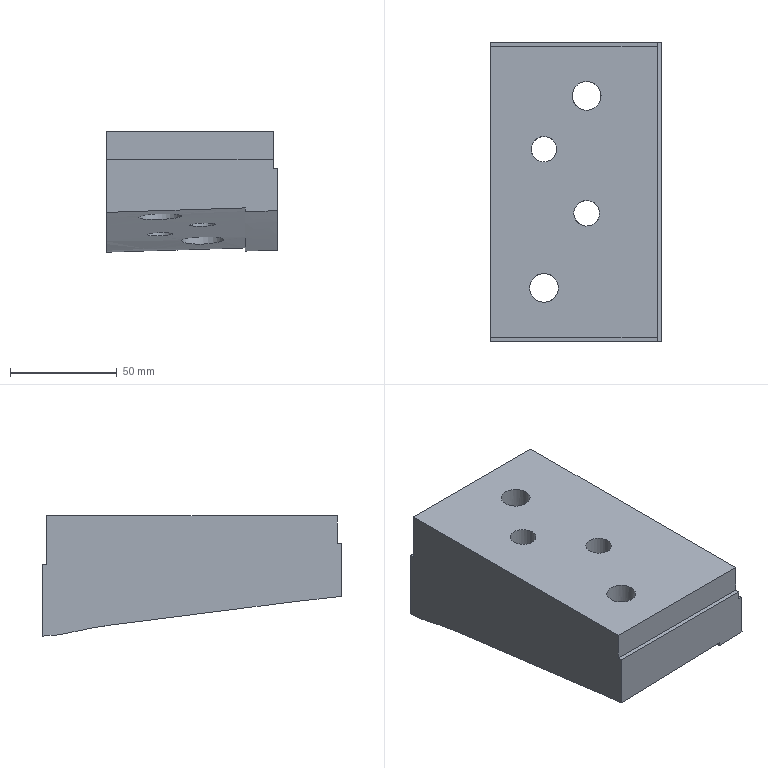Part | NX | features solid 2 | 1 solid | 22 faces | box 80 x 140 x 56.387 mm | volume 462512 mm3 | plane 9 | spline 7 | cylinder 6 | commonest cylinder face diameters 12 x2 13.5 x2 20 x2
STEP:
#1=CARTESIAN_POINT('',(-340.604,272.143,-48.935));
#2=VERTEX_POINT('',#1);
#3=CARTESIAN_POINT('',(-337.704,276.084,-49.337));
#4=CARTESIAN_POINT('',(-341.213,272.366,-48.983));
#5=CARTESIAN_POINT('',(-341.071,267.308,-48.342));
#6=CARTESIAN_POINT('',(-337.412,263.802,-47.781));
#7=CARTESIAN_POINT('',(-332.295,263.917,-47.63));
#8=CARTESIAN_POINT('',(-328.79,267.632,-47.987));
#9=CARTESIAN_POINT('',(-328.926,272.684,-48.627));
#10=CARTESIAN_POINT('',(-332.584,276.197,-49.186));
#11=CARTESIAN_POINT('',(-337.704,276.084,-49.337));
#12=CARTESIAN_POINT('',(-341.213,272.366,-48.983));
#13=CARTESIAN_POINT('',(-341.071,267.308,-48.342));
#14=B_SPLINE_CURVE_WITH_KNOTS('',3,(#3,#4,#5,#6,#7,#8,#9,#10,#11,#12,#13),.UNSPECIFIED.,.T.,.F.,(1,1,1,1,1,1,1,1,1,1,1,1,1,1,1),(-0.01413,-0.009417,-0.004708,0.,0.004708,0.009417,0.01413,0.01883,0.02354,0.02825,0.03296,0.03767,0.04238,0.04708,0.05179),.UNSPECIFIED.);
#15=EDGE_CURVE('',#2,#2,#14,.T.);
#16=ORIENTED_EDGE('',*,*,#15,.T.);
#17=EDGE_LOOP('',(#16));
#18=FACE_BOUND('',#17,.T.);
#19=CARTESIAN_POINT('',(-364.93,233.823,-44.972));
#20=VERTEX_POINT('',#19);
#21=CARTESIAN_POINT('',(-361.894,226.328,-43.775));
#22=CARTESIAN_POINT('',(-365.992,233.692,-45.025));
#23=CARTESIAN_POINT('',(-363.722,241.842,-45.959));
#24=CARTESIAN_POINT('',(-356.292,246.019,-46.2));
#25=CARTESIAN_POINT('',(-348.103,243.675,-45.634));
#26=CARTESIAN_POINT('',(-344.008,236.287,-44.614));
#27=CARTESIAN_POINT('',(-346.274,228.169,-43.516));
#28=CARTESIAN_POINT('',(-353.707,223.978,-43.211));
#29=CARTESIAN_POINT('',(-361.894,226.328,-43.775));
#30=CARTESIAN_POINT('',(-365.992,233.692,-45.025));
#31=CARTESIAN_POINT('',(-363.722,241.842,-45.959));
#32=B_SPLINE_CURVE_WITH_KNOTS('',3,(#21,#22,#23,#24,#25,#26,#27,#28,#29,#30,#31),.UNSPECIFIED.,.T.,.F.,(1,1,1,1,1,1,1,1,1,1,1,1,1,1,1),(-0.02356,-0.0157,-0.007852,0.,0.007852,0.0157,0.02356,0.03141,0.03926,0.04711,0.05496,0.06281,0.07067,0.07852,0.08637),.UNSPECIFIED.);
#33=EDGE_CURVE('',#20,#20,#32,.T.);
#34=ORIENTED_EDGE('',*,*,#33,.F.);
#35=EDGE_LOOP('',(#34));
#36=FACE_BOUND('',#35,.T.);
#37=CARTESIAN_POINT('',(-314.991,210.,-40.636));
#38=VERTEX_POINT('',#37);
#39=CARTESIAN_POINT('',(-380.,210.,-42.734));
#40=VERTEX_POINT('',#39);
#41=CARTESIAN_POINT('',(-314.991,210.,-40.636));
#42=CARTESIAN_POINT('',(-336.664,210.,-41.245));
#43=CARTESIAN_POINT('',(-358.334,210.,-41.928));
#44=CARTESIAN_POINT('',(-380.,210.,-42.734));
#45=B_SPLINE_CURVE_WITH_KNOTS('',3,(#41,#42,#43,#44),.UNSPECIFIED.,.F.,.F.,(4,4),(0.01025,0.07529),.UNSPECIFIED.);
#46=EDGE_CURVE('',#38,#40,#45,.T.);
#47=ORIENTED_EDGE('',*,*,#46,.T.);
#48=CARTESIAN_POINT('',(-380.,350.,-61.387));
#49=VERTEX_POINT('',#48);
#50=CARTESIAN_POINT('',(-380.,210.,-42.734));
#51=CARTESIAN_POINT('',(-380.,212.923,-43.037));
#52=CARTESIAN_POINT('',(-380.,218.777,-43.562));
#53=CARTESIAN_POINT('',(-380.,227.539,-44.553));
#54=CARTESIAN_POINT('',(-380.,236.272,-45.886));
#55=CARTESIAN_POINT('',(-380.,245.041,-46.917));
#56=CARTESIAN_POINT('',(-380.,253.807,-47.989));
#57=CARTESIAN_POINT('',(-380.,265.486,-49.471));
#58=CARTESIAN_POINT('',(-380.,280.086,-51.318));
#59=CARTESIAN_POINT('',(-380.,294.685,-53.165));
#60=CARTESIAN_POINT('',(-380.,306.364,-54.652));
#61=CARTESIAN_POINT('',(-380.,315.123,-55.762));
#62=CARTESIAN_POINT('',(-380.,323.875,-56.931));
#63=CARTESIAN_POINT('',(-380.,332.562,-58.574));
#64=CARTESIAN_POINT('',(-380.,341.152,-60.922));
#65=CARTESIAN_POINT('',(-380.,347.062,-61.148));
#66=CARTESIAN_POINT('',(-380.,350.,-61.387));
#67=B_SPLINE_CURVE_WITH_KNOTS('',3,(#50,#51,#52,#53,#54,#55,#56,#57,#58,#59,#60,#61,#62,#63,#64,#65,#66),.UNSPECIFIED.,.F.,.F.,(4,1,1,1,1,1,1,1,1,1,1,1,1,1,4),(0.1253,0.1342,0.143,0.1518,0.1606,0.1694,0.1782,0.1959,0.2135,0.2223,0.2311,0.2399,0.2488,0.2576,0.2664),.UNSPECIFIED.);
#68=EDGE_CURVE('',#40,#49,#67,.T.);
#69=ORIENTED_EDGE('',*,*,#68,.T.);
#70=CARTESIAN_POINT('',(-314.998,350.,-59.39));
#71=VERTEX_POINT('',#70);
#72=CARTESIAN_POINT('',(-314.998,350.,-59.39));
#73=CARTESIAN_POINT('',(-336.667,350.,-59.991));
#74=CARTESIAN_POINT('',(-358.334,350.,-60.686));
#75=CARTESIAN_POINT('',(-380.,350.,-61.387));
#76=B_SPLINE_CURVE_WITH_KNOTS('',3,(#72,#73,#74,#75),.UNSPECIFIED.,.F.,.F.,(4,4),(-0.01501,0.05002),.UNSPECIFIED.);
#77=EDGE_CURVE('',#71,#49,#76,.T.);
#78=ORIENTED_EDGE('',*,*,#77,.F.);
#79=CARTESIAN_POINT('',(-314.998,350.,-59.39));
#80=CARTESIAN_POINT('',(-314.996,347.092,-58.943));
#81=CARTESIAN_POINT('',(-314.993,341.269,-58.09));
#82=CARTESIAN_POINT('',(-314.99,332.599,-56.409));
#83=CARTESIAN_POINT('',(-314.988,323.924,-54.761));
#84=CARTESIAN_POINT('',(-314.986,315.176,-53.571));
#85=CARTESIAN_POINT('',(-314.985,306.414,-52.466));
#86=CARTESIAN_POINT('',(-314.983,294.733,-50.983));
#87=CARTESIAN_POINT('',(-314.983,280.132,-49.135));
#88=CARTESIAN_POINT('',(-314.984,262.608,-46.929));
#89=CARTESIAN_POINT('',(-314.985,248.007,-45.079));
#90=CARTESIAN_POINT('',(-314.987,236.316,-43.671));
#91=CARTESIAN_POINT('',(-314.988,227.574,-42.418));
#92=CARTESIAN_POINT('',(-314.99,218.799,-41.409));
#93=CARTESIAN_POINT('',(-314.991,212.932,-40.901));
#94=CARTESIAN_POINT('',(-314.991,210.,-40.636));
#95=B_SPLINE_CURVE_WITH_KNOTS('',3,(#79,#80,#81,#82,#83,#84,#85,#86,#87,#88,#89,#90,#91,#92,#93,#94),.UNSPECIFIED.,.F.,.F.,(4,1,1,1,1,1,1,1,1,1,1,1,1,4),(0.,0.008827,0.01765,0.02648,0.03531,0.04413,0.05296,0.07061,0.08827,0.1059,0.1147,0.1236,0.1324,0.1412),.UNSPECIFIED.);
#96=EDGE_CURVE('',#71,#38,#95,.T.);
#97=ORIENTED_EDGE('',*,*,#96,.T.);
#98=EDGE_LOOP('',(#47,#69,#78,#97));
#99=FACE_BOUND('',#98,.T.);
#100=CARTESIAN_POINT('',(-360.605,302.142,-53.408));
#101=VERTEX_POINT('',#100);
#102=CARTESIAN_POINT('',(-357.705,306.084,-53.808));
#103=CARTESIAN_POINT('',(-361.213,302.365,-53.457));
#104=CARTESIAN_POINT('',(-361.07,297.307,-52.812));
#105=CARTESIAN_POINT('',(-357.411,293.802,-52.241));
#106=CARTESIAN_POINT('',(-352.295,293.917,-52.079));
#107=CARTESIAN_POINT('',(-348.789,297.634,-52.43));
#108=CARTESIAN_POINT('',(-348.927,302.686,-53.074));
#109=CARTESIAN_POINT('',(-352.585,306.197,-53.646));
#110=CARTESIAN_POINT('',(-357.705,306.084,-53.808));
#111=CARTESIAN_POINT('',(-361.213,302.365,-53.457));
#112=CARTESIAN_POINT('',(-361.07,297.307,-52.812));
#113=B_SPLINE_CURVE_WITH_KNOTS('',3,(#102,#103,#104,#105,#106,#107,#108,#109,#110,#111,#112),.UNSPECIFIED.,.T.,.F.,(1,1,1,1,1,1,1,1,1,1,1,1,1,1,1),(-0.01413,-0.009418,-0.004709,0.,0.004709,0.009418,0.01413,0.01884,0.02354,0.02825,0.03296,0.03767,0.04238,0.04709,0.0518),.UNSPECIFIED.);
#114=EDGE_CURVE('',#101,#101,#113,.T.);
#115=ORIENTED_EDGE('',*,*,#114,.T.);
#116=EDGE_LOOP('',(#115));
#117=FACE_BOUND('',#116,.T.);
#118=CARTESIAN_POINT('',(-325.086,326.305,-55.559));
#119=VERTEX_POINT('',#118);
#120=CARTESIAN_POINT('',(-328.189,333.733,-57.085));
#121=CARTESIAN_POINT('',(-324.036,326.454,-55.489));
#122=CARTESIAN_POINT('',(-326.178,318.281,-54.313));
#123=CARTESIAN_POINT('',(-333.578,313.989,-54.013));
#124=CARTESIAN_POINT('',(-341.824,316.259,-54.566));
#125=CARTESIAN_POINT('',(-345.974,323.624,-55.697));
#126=CARTESIAN_POINT('',(-343.806,331.716,-57.207));
#127=CARTESIAN_POINT('',(-336.422,336.014,-57.861));
#128=CARTESIAN_POINT('',(-328.189,333.733,-57.085));
#129=CARTESIAN_POINT('',(-324.036,326.454,-55.489));
#130=CARTESIAN_POINT('',(-326.178,318.281,-54.313));
#131=B_SPLINE_CURVE_WITH_KNOTS('',3,(#120,#121,#122,#123,#124,#125,#126,#127,#128,#129,#130),.UNSPECIFIED.,.T.,.F.,(1,1,1,1,1,1,1,1,1,1,1,1,1,1,1),(-0.02362,-0.01575,-0.007874,0.,0.007874,0.01575,0.02362,0.0315,0.03937,0.04725,0.05512,0.063,0.07087,0.07874,0.08662),.UNSPECIFIED.);
#132=EDGE_CURVE('',#119,#119,#131,.T.);
#133=ORIENTED_EDGE('',*,*,#132,.F.);
#134=EDGE_LOOP('',(#133));
#135=FACE_BOUND('',#134,.T.);
#136=CARTESIAN_POINT('',(-300.962,350.,-59.01));
#137=CARTESIAN_POINT('',(-301.431,346.762,-58.489));
#138=CARTESIAN_POINT('',(-302.299,340.897,-57.565));
#139=CARTESIAN_POINT('',(-303.25,332.345,-55.971));
#140=CARTESIAN_POINT('',(-304.418,323.079,-54.303));
#141=CARTESIAN_POINT('',(-305.393,313.774,-53.112));
#142=CARTESIAN_POINT('',(-306.505,303.143,-51.799));
#143=CARTESIAN_POINT('',(-307.441,293.837,-50.646));
#144=CARTESIAN_POINT('',(-308.479,283.202,-49.331));
#145=CARTESIAN_POINT('',(-309.382,273.894,-48.18));
#146=CARTESIAN_POINT('',(-310.372,263.256,-46.87));
#147=CARTESIAN_POINT('',(-311.258,253.944,-45.722));
#148=CARTESIAN_POINT('',(-312.072,243.308,-44.419));
#149=CARTESIAN_POINT('',(-312.85,233.989,-43.303));
#150=CARTESIAN_POINT('',(-313.651,223.335,-41.796));
#151=CARTESIAN_POINT('',(-314.257,215.772,-41.146));
#152=CARTESIAN_POINT('',(-314.465,210.889,-40.701));
#153=CARTESIAN_POINT('',(-314.5,210.,-40.622));
#154=CARTESIAN_POINT('',(-314.02,350.,-59.356));
#155=CARTESIAN_POINT('',(-314.503,346.762,-58.865));
#156=CARTESIAN_POINT('',(-315.396,340.897,-58.023));
#157=CARTESIAN_POINT('',(-316.39,332.345,-56.402));
#158=CARTESIAN_POINT('',(-317.606,323.079,-54.671));
#159=CARTESIAN_POINT('',(-318.618,313.774,-53.501));
#160=CARTESIAN_POINT('',(-319.775,303.143,-52.185));
#161=CARTESIAN_POINT('',(-320.748,293.837,-51.037));
#162=CARTESIAN_POINT('',(-321.828,283.202,-49.725));
#163=CARTESIAN_POINT('',(-322.766,273.894,-48.577));
#164=CARTESIAN_POINT('',(-323.796,263.256,-47.271));
#165=CARTESIAN_POINT('',(-324.709,253.944,-46.126));
#166=CARTESIAN_POINT('',(-325.587,243.308,-44.837));
#167=CARTESIAN_POINT('',(-326.387,233.989,-43.734));
#168=CARTESIAN_POINT('',(-327.225,223.335,-42.178));
#169=CARTESIAN_POINT('',(-327.854,215.772,-41.548));
#170=CARTESIAN_POINT('',(-328.077,210.889,-41.086));
#171=CARTESIAN_POINT('',(-328.115,210.,-41.004));
#172=CARTESIAN_POINT('',(-340.52,350.,-60.099));
#173=CARTESIAN_POINT('',(-341.03,346.762,-59.688));
#174=CARTESIAN_POINT('',(-341.969,340.897,-59.065));
#175=CARTESIAN_POINT('',(-343.058,332.345,-57.312));
#176=CARTESIAN_POINT('',(-344.37,323.079,-55.476));
#177=CARTESIAN_POINT('',(-345.46,313.774,-54.346));
#178=CARTESIAN_POINT('',(-346.706,303.143,-53.023));
#179=CARTESIAN_POINT('',(-347.754,293.837,-51.885));
#180=CARTESIAN_POINT('',(-348.919,283.202,-50.579));
#181=CARTESIAN_POINT('',(-349.928,273.894,-49.435));
#182=CARTESIAN_POINT('',(-351.041,263.256,-48.137));
#183=CARTESIAN_POINT('',(-352.009,253.944,-46.994));
#184=CARTESIAN_POINT('',(-353.015,243.308,-45.734));
#185=CARTESIAN_POINT('',(-353.86,233.989,-44.657));
#186=CARTESIAN_POINT('',(-354.774,223.335,-43.011));
#187=CARTESIAN_POINT('',(-355.446,215.772,-42.425));
#188=CARTESIAN_POINT('',(-355.703,210.889,-41.926));
#189=CARTESIAN_POINT('',(-355.748,210.,-41.838));
#190=CARTESIAN_POINT('',(-367.021,350.,-60.967));
#191=CARTESIAN_POINT('',(-367.548,346.762,-60.703));
#192=CARTESIAN_POINT('',(-368.502,340.897,-60.466));
#193=CARTESIAN_POINT('',(-369.739,332.345,-58.166));
#194=CARTESIAN_POINT('',(-371.126,323.079,-56.442));
#195=CARTESIAN_POINT('',(-372.298,313.774,-55.304));
#196=CARTESIAN_POINT('',(-373.633,303.143,-53.988));
#197=CARTESIAN_POINT('',(-374.757,293.837,-52.856));
#198=CARTESIAN_POINT('',(-376.006,283.202,-51.554));
#199=CARTESIAN_POINT('',(-377.086,273.894,-50.413));
#200=CARTESIAN_POINT('',(-378.28,263.256,-49.117));
#201=CARTESIAN_POINT('',(-379.311,253.944,-47.967));
#202=CARTESIAN_POINT('',(-380.416,243.308,-46.721));
#203=CARTESIAN_POINT('',(-381.319,233.989,-45.631));
#204=CARTESIAN_POINT('',(-382.302,223.335,-44.011));
#205=CARTESIAN_POINT('',(-383.015,215.772,-43.446));
#206=CARTESIAN_POINT('',(-383.311,210.889,-42.932));
#207=CARTESIAN_POINT('',(-383.363,210.,-42.841));
#208=CARTESIAN_POINT('',(-380.472,350.,-61.402));
#209=CARTESIAN_POINT('',(-381.011,346.762,-61.156));
#210=CARTESIAN_POINT('',(-381.985,340.897,-60.965));
#211=CARTESIAN_POINT('',(-383.269,332.345,-58.644));
#212=CARTESIAN_POINT('',(-384.699,323.079,-56.959));
#213=CARTESIAN_POINT('',(-385.911,313.774,-55.824));
#214=CARTESIAN_POINT('',(-387.291,303.143,-54.514));
#215=CARTESIAN_POINT('',(-388.453,293.837,-53.383));
#216=CARTESIAN_POINT('',(-389.745,283.202,-52.084));
#217=CARTESIAN_POINT('',(-390.861,273.894,-50.942));
#218=CARTESIAN_POINT('',(-392.096,263.256,-49.645));
#219=CARTESIAN_POINT('',(-393.163,253.944,-48.489));
#220=CARTESIAN_POINT('',(-394.303,243.308,-47.245));
#221=CARTESIAN_POINT('',(-395.243,233.989,-46.127));
#222=CARTESIAN_POINT('',(-396.256,223.335,-44.574));
#223=CARTESIAN_POINT('',(-396.988,215.772,-44.006));
#224=CARTESIAN_POINT('',(-397.308,210.889,-43.498));
#225=CARTESIAN_POINT('',(-397.364,210.,-43.407));
#226=B_SPLINE_SURFACE_WITH_KNOTS('',3,3,((#136,#137,#138,#139,#140,#141,#142,#143,#144,#145,#146,#147,#148,#149,#150,#151,#152,#153),(#154,#155,#156,#157,#158,#159,#160,#161,#162,#163,#164,#165,#166,#167,#168,#169,#170,#171),(#172,#173,#174,#175,#176,#177,#178,#179,#180,#181,#182,#183,#184,#185,#186,#187,#188,#189),(#190,#191,#192,#193,#194,#195,#196,#197,#198,#199,#200,#201,#202,#203,#204,#205,#206,#207),(#208,#209,#210,#211,#212,#213,#214,#215,#216,#217,#218,#219,#220,#221,#222,#223,#224,#225)),.UNSPECIFIED.,.F.,.F.,.F.,(4,1,4),(4,1,1,1,1,1,1,1,1,1,1,1,1,1,1,4),(0.7767,0.8125,0.8494),(0.2465,0.2656,0.2812,0.2969,0.3203,0.3359,0.3594,0.375,0.3984,0.4141,0.4375,0.4531,0.4766,0.4922,0.5156,0.5208),.UNSPECIFIED.);
#227=ADVANCED_FACE('',(#18,#36,#99,#117,#135),#226,.F.);
#228=CARTESIAN_POINT('',(-302.,348.,-28.));
#229=VERTEX_POINT('',#228);
#230=CARTESIAN_POINT('',(-380.,348.,-28.));
#231=VERTEX_POINT('',#230);
#232=CARTESIAN_POINT('',(-302.,348.,-28.));
#233=DIRECTION('',(1.,0.,0.));
#234=VECTOR('',#233,1000.);
#235=LINE('',#232,#234);
#236=EDGE_CURVE('',#229,#231,#235,.F.);
#237=ORIENTED_EDGE('',*,*,#236,.F.);
#238=CARTESIAN_POINT('',(-302.,350.,-28.));
#239=VERTEX_POINT('',#238);
#240=CARTESIAN_POINT('',(-302.,350.,-28.));
#241=DIRECTION('',(0.,1.,0.));
#242=VECTOR('',#241,1000.);
#243=LINE('',#240,#242);
#244=EDGE_CURVE('',#239,#229,#243,.F.);
#245=ORIENTED_EDGE('',*,*,#244,.F.);
#246=CARTESIAN_POINT('',(-380.,350.,-28.));
#247=VERTEX_POINT('',#246);
#248=CARTESIAN_POINT('',(-302.,350.,-28.));
#249=DIRECTION('',(1.,0.,0.));
#250=VECTOR('',#249,1000.);
#251=LINE('',#248,#250);
#252=EDGE_CURVE('',#239,#247,#251,.F.);
#253=ORIENTED_EDGE('',*,*,#252,.T.);
#254=CARTESIAN_POINT('',(-380.,350.,-28.));
#255=DIRECTION('',(0.,1.,0.));
#256=VECTOR('',#255,1000.);
#257=LINE('',#254,#256);
#258=EDGE_CURVE('',#247,#231,#257,.F.);
#259=ORIENTED_EDGE('',*,*,#258,.T.);
#260=EDGE_LOOP('',(#237,#245,#253,#259));
#261=FACE_BOUND('',#260,.T.);
#262=CARTESIAN_POINT('',(-302.,350.,-28.));
#263=DIRECTION('',(0.,0.,1.));
#264=DIRECTION('',(1.,0.,0.));
#265=AXIS2_PLACEMENT_3D('',#262,#263,#264);
#266=PLANE('',#265);
#267=ADVANCED_FACE('',(#261),#266,.T.);
#268=CARTESIAN_POINT('',(-380.,350.,-61.387));
#269=CARTESIAN_POINT('',(-380.,350.,-50.258));
#270=CARTESIAN_POINT('',(-380.,350.,-39.129));
#271=CARTESIAN_POINT('',(-380.,350.,-28.));
#272=B_SPLINE_CURVE_WITH_KNOTS('',3,(#268,#269,#270,#271),.UNSPECIFIED.,.F.,.F.,(4,4),(0.,0.03339),.UNSPECIFIED.);
#273=EDGE_CURVE('',#49,#247,#272,.T.);
#274=ORIENTED_EDGE('',*,*,#273,.T.);
#275=ORIENTED_EDGE('',*,*,#252,.F.);
#276=CARTESIAN_POINT('',(-302.,350.,-40.416));
#277=VERTEX_POINT('',#276);
#278=CARTESIAN_POINT('',(-302.,350.,-40.416));
#279=DIRECTION('',(0.,0.,1.));
#280=VECTOR('',#279,1000.);
#281=LINE('',#278,#280);
#282=EDGE_CURVE('',#277,#239,#281,.T.);
#283=ORIENTED_EDGE('',*,*,#282,.F.);
#284=CARTESIAN_POINT('',(-300.,350.,-40.416));
#285=VERTEX_POINT('',#284);
#286=CARTESIAN_POINT('',(-302.,350.,-40.416));
#287=CARTESIAN_POINT('',(-301.333,350.,-40.416));
#288=CARTESIAN_POINT('',(-300.667,350.,-40.416));
#289=CARTESIAN_POINT('',(-300.,350.,-40.416));
#290=B_SPLINE_CURVE_WITH_KNOTS('',3,(#286,#287,#288,#289),.UNSPECIFIED.,.F.,.F.,(4,4),(0.,1.),.UNSPECIFIED.);
#291=EDGE_CURVE('',#285,#277,#290,.F.);
#292=ORIENTED_EDGE('',*,*,#291,.F.);
#293=CARTESIAN_POINT('',(-300.,350.,-60.416));
#294=VERTEX_POINT('',#293);
#295=CARTESIAN_POINT('',(-300.,350.,-38.122));
#296=DIRECTION('',(0.,0.,1.));
#297=VECTOR('',#296,1000.);
#298=LINE('',#295,#297);
#299=EDGE_CURVE('',#294,#285,#298,.T.);
#300=ORIENTED_EDGE('',*,*,#299,.F.);
#301=CARTESIAN_POINT('',(-314.998,350.,-60.862));
#302=VERTEX_POINT('',#301);
#303=CARTESIAN_POINT('',(-314.998,350.,-60.862));
#304=CARTESIAN_POINT('',(-309.999,350.,-60.709));
#305=CARTESIAN_POINT('',(-304.999,350.,-60.561));
#306=CARTESIAN_POINT('',(-300.,350.,-60.416));
#307=B_SPLINE_CURVE_WITH_KNOTS('',3,(#303,#304,#305,#306),.UNSPECIFIED.,.F.,.F.,(4,4),(0.02527,0.04027),.UNSPECIFIED.);
#308=EDGE_CURVE('',#302,#294,#307,.T.);
#309=ORIENTED_EDGE('',*,*,#308,.F.);
#310=CARTESIAN_POINT('',(-314.998,350.,-96.));
#311=DIRECTION('',(0.,0.,1.));
#312=VECTOR('',#311,1000.);
#313=LINE('',#310,#312);
#314=EDGE_CURVE('',#302,#71,#313,.T.);
#315=ORIENTED_EDGE('',*,*,#314,.T.);
#316=ORIENTED_EDGE('',*,*,#77,.T.);
#317=EDGE_LOOP('',(#274,#275,#283,#292,#300,#309,#315,#316));
#318=FACE_BOUND('',#317,.T.);
#319=CARTESIAN_POINT('',(440.921,350.,-40.306));
#320=DIRECTION('',(0.,1.,0.));
#321=DIRECTION('',(0.,0.,1.));
#322=AXIS2_PLACEMENT_3D('',#319,#320,#321);
#323=PLANE('',#322);
#324=ADVANCED_FACE('',(#318),#323,.T.);
#325=CARTESIAN_POINT('',(-302.,348.,-5.));
#326=VERTEX_POINT('',#325);
#327=CARTESIAN_POINT('',(-302.,348.,12.));
#328=DIRECTION('',(0.,0.,1.));
#329=VECTOR('',#328,1000.);
#330=LINE('',#327,#329);
#331=EDGE_CURVE('',#326,#229,#330,.F.);
#332=ORIENTED_EDGE('',*,*,#331,.T.);
#333=ORIENTED_EDGE('',*,*,#236,.T.);
#334=CARTESIAN_POINT('',(-380.,348.,-5.));
#335=VERTEX_POINT('',#334);
#336=CARTESIAN_POINT('',(-380.,348.,12.));
#337=DIRECTION('',(0.,0.,1.));
#338=VECTOR('',#337,1000.);
#339=LINE('',#336,#338);
#340=EDGE_CURVE('',#335,#231,#339,.F.);
#341=ORIENTED_EDGE('',*,*,#340,.F.);
#342=CARTESIAN_POINT('',(-302.,348.,-5.));
#343=DIRECTION('',(-1.,0.,0.));
#344=VECTOR('',#343,1000.);
#345=LINE('',#342,#344);
#346=EDGE_CURVE('',#326,#335,#345,.T.);
#347=ORIENTED_EDGE('',*,*,#346,.F.);
#348=EDGE_LOOP('',(#332,#333,#341,#347));
#349=FACE_BOUND('',#348,.T.);
#350=CARTESIAN_POINT('',(-302.,348.,12.));
#351=DIRECTION('',(0.,1.,0.));
#352=DIRECTION('',(-1.,0.,0.));
#353=AXIS2_PLACEMENT_3D('',#350,#351,#352);
#354=PLANE('',#353);
#355=ADVANCED_FACE('',(#349),#354,.T.);
#356=CARTESIAN_POINT('',(-329.,270.,-5.));
#357=VERTEX_POINT('',#356);
#358=CARTESIAN_POINT('',(-335.,270.,-5.));
#359=DIRECTION('',(0.,0.,1.));
#360=DIRECTION('',(1.,0.,0.));
#361=AXIS2_PLACEMENT_3D('',#358,#359,#360);
#362=CIRCLE('',#361,6.);
#363=EDGE_CURVE('',#357,#357,#362,.F.);
#364=ORIENTED_EDGE('',*,*,#363,.T.);
#365=EDGE_LOOP('',(#364));
#366=FACE_BOUND('',#365,.T.);
#367=CARTESIAN_POINT('',(-341.75,325.,-5.));
#368=VERTEX_POINT('',#367);
#369=CARTESIAN_POINT('',(-335.,325.,-5.));
#370=DIRECTION('',(0.,0.,-1.));
#371=DIRECTION('',(-1.,0.,0.));
#372=AXIS2_PLACEMENT_3D('',#369,#370,#371);
#373=CIRCLE('',#372,6.75);
#374=EDGE_CURVE('',#368,#368,#373,.T.);
#375=ORIENTED_EDGE('',*,*,#374,.T.);
#376=EDGE_LOOP('',(#375));
#377=FACE_BOUND('',#376,.T.);
#378=CARTESIAN_POINT('',(-349.,300.,-5.));
#379=VERTEX_POINT('',#378);
#380=CARTESIAN_POINT('',(-355.,300.,-5.));
#381=DIRECTION('',(0.,0.,1.));
#382=DIRECTION('',(1.,0.,0.));
#383=AXIS2_PLACEMENT_3D('',#380,#381,#382);
#384=CIRCLE('',#383,6.);
#385=EDGE_CURVE('',#379,#379,#384,.F.);
#386=ORIENTED_EDGE('',*,*,#385,.T.);
#387=EDGE_LOOP('',(#386));
#388=FACE_BOUND('',#387,.T.);
#389=CARTESIAN_POINT('',(-361.75,235.,-5.));
#390=VERTEX_POINT('',#389);
#391=CARTESIAN_POINT('',(-355.,235.,-5.));
#392=DIRECTION('',(0.,0.,-1.));
#393=DIRECTION('',(-1.,0.,0.));
#394=AXIS2_PLACEMENT_3D('',#391,#392,#393);
#395=CIRCLE('',#394,6.75);
#396=EDGE_CURVE('',#390,#390,#395,.T.);
#397=ORIENTED_EDGE('',*,*,#396,.T.);
#398=EDGE_LOOP('',(#397));
#399=FACE_BOUND('',#398,.T.);
#400=CARTESIAN_POINT('',(-380.,212.,-5.));
#401=VERTEX_POINT('',#400);
#402=CARTESIAN_POINT('',(-302.,212.,-5.));
#403=VERTEX_POINT('',#402);
#404=CARTESIAN_POINT('',(0.,212.,-5.));
#405=DIRECTION('',(-1.,0.,0.));
#406=VECTOR('',#405,1000.);
#407=LINE('',#404,#406);
#408=EDGE_CURVE('',#401,#403,#407,.F.);
#409=ORIENTED_EDGE('',*,*,#408,.T.);
#410=CARTESIAN_POINT('',(-302.,348.,-5.));
#411=CARTESIAN_POINT('',(-302.,302.667,-5.));
#412=CARTESIAN_POINT('',(-302.,257.333,-5.));
#413=CARTESIAN_POINT('',(-302.,212.,-5.));
#414=B_SPLINE_CURVE_WITH_KNOTS('',3,(#410,#411,#412,#413),.UNSPECIFIED.,.F.,.F.,(4,4),(1.054,1.19),.UNSPECIFIED.);
#415=EDGE_CURVE('',#326,#403,#414,.T.);
#416=ORIENTED_EDGE('',*,*,#415,.F.);
#417=ORIENTED_EDGE('',*,*,#346,.T.);
#418=CARTESIAN_POINT('',(-380.,212.,-5.));
#419=CARTESIAN_POINT('',(-380.,257.333,-5.));
#420=CARTESIAN_POINT('',(-380.,302.667,-5.));
#421=CARTESIAN_POINT('',(-380.,348.,-5.));
#422=B_SPLINE_CURVE_WITH_KNOTS('',3,(#418,#419,#420,#421),.UNSPECIFIED.,.F.,.F.,(4,4),(0.,0.136),.UNSPECIFIED.);
#423=EDGE_CURVE('',#401,#335,#422,.T.);
#424=ORIENTED_EDGE('',*,*,#423,.F.);
#425=EDGE_LOOP('',(#409,#416,#417,#424));
#426=FACE_BOUND('',#425,.T.);
#427=CARTESIAN_POINT('',(0.,0.,-5.));
#428=DIRECTION('',(0.,0.,1.));
#429=DIRECTION('',(-1.,0.,0.));
#430=AXIS2_PLACEMENT_3D('',#427,#428,#429);
#431=PLANE('',#430);
#432=ADVANCED_FACE('',(#366,#377,#388,#399,#426),#431,.T.);
#433=CARTESIAN_POINT('',(-300.,210.,-21.967));
#434=VERTEX_POINT('',#433);
#435=CARTESIAN_POINT('',(-300.,210.,-21.967));
#436=CARTESIAN_POINT('',(-300.,256.574,-26.699));
#437=CARTESIAN_POINT('',(-300.,303.268,-32.848));
#438=CARTESIAN_POINT('',(-300.,350.,-40.416));
#439=B_SPLINE_CURVE_WITH_KNOTS('',3,(#435,#436,#437,#438),.UNSPECIFIED.,.F.,.F.,(4,4),(0.4701,1.),.UNSPECIFIED.);
#440=EDGE_CURVE('',#434,#285,#439,.T.);
#441=ORIENTED_EDGE('',*,*,#440,.T.);
#442=ORIENTED_EDGE('',*,*,#291,.T.);
#443=CARTESIAN_POINT('',(-302.,210.,-21.967));
#444=VERTEX_POINT('',#443);
#445=CARTESIAN_POINT('',(-302.,350.,-40.416));
#446=CARTESIAN_POINT('',(-302.,303.548,-32.894));
#447=CARTESIAN_POINT('',(-302.,256.829,-26.725));
#448=CARTESIAN_POINT('',(-302.,210.,-21.967));
#449=B_SPLINE_CURVE_WITH_KNOTS('',3,(#445,#446,#447,#448),.UNSPECIFIED.,.F.,.F.,(4,4),(0.,0.5298),.UNSPECIFIED.);
#450=EDGE_CURVE('',#444,#277,#449,.F.);
#451=ORIENTED_EDGE('',*,*,#450,.F.);
#452=CARTESIAN_POINT('',(-300.,210.,-21.967));
#453=CARTESIAN_POINT('',(-300.667,210.,-21.967));
#454=CARTESIAN_POINT('',(-301.333,210.,-21.967));
#455=CARTESIAN_POINT('',(-302.,210.,-21.967));
#456=B_SPLINE_CURVE_WITH_KNOTS('',3,(#452,#453,#454,#455),.UNSPECIFIED.,.F.,.F.,(4,4),(0.,0.002),.UNSPECIFIED.);
#457=EDGE_CURVE('',#434,#444,#456,.T.);
#458=ORIENTED_EDGE('',*,*,#457,.F.);
#459=EDGE_LOOP('',(#441,#442,#451,#458));
#460=FACE_BOUND('',#459,.T.);
#461=CARTESIAN_POINT('',(-302.,210.,-21.967));
#462=CARTESIAN_POINT('',(-302.,212.63,-22.234));
#463=CARTESIAN_POINT('',(-302.,215.26,-22.506));
#464=CARTESIAN_POINT('',(-302.,262.074,-27.421));
#465=CARTESIAN_POINT('',(-302.,306.157,-33.316));
#466=CARTESIAN_POINT('',(-302.,350.,-40.416));
#467=CARTESIAN_POINT('',(-300.,210.,-21.967));
#468=CARTESIAN_POINT('',(-300.,212.63,-22.234));
#469=CARTESIAN_POINT('',(-300.,215.26,-22.506));
#470=CARTESIAN_POINT('',(-300.,262.074,-27.421));
#471=CARTESIAN_POINT('',(-300.,306.157,-33.316));
#472=CARTESIAN_POINT('',(-300.,350.,-40.416));
#473=B_SPLINE_SURFACE_WITH_KNOTS('',1,3,((#461,#462,#463,#464,#465,#466),(#467,#468,#469,#470,#471,#472)),.SURF_OF_LINEAR_EXTRUSION.,.F.,.F.,.F.,(2,2),(4,2,4),(0.,1.),(0.4702,0.5,1.),.UNSPECIFIED.);
#474=ADVANCED_FACE('',(#460),#473,.T.);
#475=ORIENTED_EDGE('',*,*,#96,.F.);
#476=ORIENTED_EDGE('',*,*,#314,.F.);
#477=CARTESIAN_POINT('',(-314.991,210.,-42.394));
#478=VERTEX_POINT('',#477);
#479=CARTESIAN_POINT('',(-314.998,350.,-60.862));
#480=CARTESIAN_POINT('',(-314.973,303.523,-53.327));
#481=CARTESIAN_POINT('',(-314.983,256.834,-47.158));
#482=CARTESIAN_POINT('',(-314.991,210.,-42.394));
#483=B_SPLINE_CURVE_WITH_KNOTS('',3,(#479,#480,#481,#482),.UNSPECIFIED.,.F.,.F.,(4,4),(0.,0.1412),.UNSPECIFIED.);
#484=EDGE_CURVE('',#302,#478,#483,.T.);
#485=ORIENTED_EDGE('',*,*,#484,.T.);
#486=CARTESIAN_POINT('',(-314.991,210.,-46.286));
#487=DIRECTION('',(0.,0.,1.));
#488=VECTOR('',#487,1000.);
#489=LINE('',#486,#488);
#490=EDGE_CURVE('',#38,#478,#489,.F.);
#491=ORIENTED_EDGE('',*,*,#490,.F.);
#492=EDGE_LOOP('',(#475,#476,#485,#491));
#493=FACE_BOUND('',#492,.T.);
#494=CARTESIAN_POINT('',(-314.991,210.,-60.983));
#495=CARTESIAN_POINT('',(-314.991,210.,-40.514));
#496=CARTESIAN_POINT('',(-314.991,211.512,-60.983));
#497=CARTESIAN_POINT('',(-314.991,211.512,-40.514));
#498=CARTESIAN_POINT('',(-314.991,213.411,-60.983));
#499=CARTESIAN_POINT('',(-314.991,213.411,-40.514));
#500=CARTESIAN_POINT('',(-314.99,215.673,-60.983));
#501=CARTESIAN_POINT('',(-314.99,215.673,-40.514));
#502=CARTESIAN_POINT('',(-314.99,216.645,-60.983));
#503=CARTESIAN_POINT('',(-314.99,216.645,-40.514));
#504=CARTESIAN_POINT('',(-314.99,217.355,-60.983));
#505=CARTESIAN_POINT('',(-314.99,217.355,-40.514));
#506=CARTESIAN_POINT('',(-314.99,218.314,-60.983));
#507=CARTESIAN_POINT('',(-314.99,218.314,-40.514));
#508=CARTESIAN_POINT('',(-314.989,219.979,-60.983));
#509=CARTESIAN_POINT('',(-314.989,219.979,-40.514));
#510=CARTESIAN_POINT('',(-314.989,222.347,-60.983));
#511=CARTESIAN_POINT('',(-314.989,222.347,-40.514));
#512=CARTESIAN_POINT('',(-314.988,226.104,-60.983));
#513=CARTESIAN_POINT('',(-314.988,226.104,-40.514));
#514=CARTESIAN_POINT('',(-314.988,230.745,-60.983));
#515=CARTESIAN_POINT('',(-314.988,230.745,-40.514));
#516=CARTESIAN_POINT('',(-314.987,236.223,-60.983));
#517=CARTESIAN_POINT('',(-314.987,236.223,-40.514));
#518=CARTESIAN_POINT('',(-314.986,243.407,-60.983));
#519=CARTESIAN_POINT('',(-314.986,243.407,-40.514));
#520=CARTESIAN_POINT('',(-314.984,255.663,-60.983));
#521=CARTESIAN_POINT('',(-314.984,255.663,-40.514));
#522=CARTESIAN_POINT('',(-314.982,285.554,-60.983));
#523=CARTESIAN_POINT('',(-314.982,285.554,-40.514));
#524=CARTESIAN_POINT('',(-314.985,319.631,-60.983));
#525=CARTESIAN_POINT('',(-314.985,319.631,-40.514));
#526=CARTESIAN_POINT('',(-314.993,342.011,-60.983));
#527=CARTESIAN_POINT('',(-314.993,342.011,-40.514));
#528=CARTESIAN_POINT('',(-314.998,350.,-60.983));
#529=CARTESIAN_POINT('',(-314.998,350.,-40.514));
#530=B_SPLINE_SURFACE_WITH_KNOTS('',3,1,((#494,#495),(#496,#497),(#498,#499),(#500,#501),(#502,#503),(#504,#505),(#506,#507),(#508,#509),(#510,#511),(#512,#513),(#514,#515),(#516,#517),(#518,#519),(#520,#521),(#522,#523),(#524,#525),(#526,#527),(#528,#529)),.UNSPECIFIED.,.F.,.F.,.F.,(4,1,1,1,1,1,1,1,1,1,1,1,1,1,1,4),(2,2),(0.4728,0.4893,0.4934,0.4975,0.4996,0.5017,0.5058,0.514,0.5222,0.5387,0.5552,0.5717,0.6046,0.6705,0.8682,1.),(0.,1.),.UNSPECIFIED.);
#531=ADVANCED_FACE('',(#493),#530,.F.);
#532=ORIENTED_EDGE('',*,*,#484,.F.);
#533=ORIENTED_EDGE('',*,*,#308,.T.);
#534=CARTESIAN_POINT('',(-300.,210.,-41.967));
#535=VERTEX_POINT('',#534);
#536=CARTESIAN_POINT('',(-300.,210.,-41.967));
#537=CARTESIAN_POINT('',(-300.,256.829,-46.725));
#538=CARTESIAN_POINT('',(-300.,303.537,-52.892));
#539=CARTESIAN_POINT('',(-300.,350.,-60.416));
#540=B_SPLINE_CURVE_WITH_KNOTS('',3,(#536,#537,#538,#539),.UNSPECIFIED.,.F.,.F.,(4,4),(0.1883,0.3295),.UNSPECIFIED.);
#541=EDGE_CURVE('',#535,#294,#540,.T.);
#542=ORIENTED_EDGE('',*,*,#541,.F.);
#543=CARTESIAN_POINT('',(-314.991,210.,-42.394));
#544=CARTESIAN_POINT('',(-309.994,210.,-42.247));
#545=CARTESIAN_POINT('',(-304.997,210.,-42.105));
#546=CARTESIAN_POINT('',(-300.,210.,-41.967));
#547=B_SPLINE_CURVE_WITH_KNOTS('',3,(#543,#544,#545,#546),.UNSPECIFIED.,.F.,.F.,(4,4),(0.0001238,0.01512),.UNSPECIFIED.);
#548=EDGE_CURVE('',#478,#535,#547,.T.);
#549=ORIENTED_EDGE('',*,*,#548,.F.);
#550=EDGE_LOOP('',(#532,#533,#542,#549));
#551=FACE_BOUND('',#550,.T.);
#552=CARTESIAN_POINT('',(-315.088,350.898,-61.011));
#553=CARTESIAN_POINT('',(-311.287,350.884,-60.892));
#554=CARTESIAN_POINT('',(-307.486,350.87,-60.776));
#555=CARTESIAN_POINT('',(-303.685,350.856,-60.662));
#556=CARTESIAN_POINT('',(-299.885,350.843,-60.55));
#557=CARTESIAN_POINT('',(-315.095,315.337,-55.233));
#558=CARTESIAN_POINT('',(-311.294,315.323,-55.116));
#559=CARTESIAN_POINT('',(-307.493,315.31,-55.001));
#560=CARTESIAN_POINT('',(-303.692,315.296,-54.888));
#561=CARTESIAN_POINT('',(-299.891,315.283,-54.778));
#562=CARTESIAN_POINT('',(-315.101,279.869,-50.193));
#563=CARTESIAN_POINT('',(-311.3,279.855,-50.077));
#564=CARTESIAN_POINT('',(-307.499,279.842,-49.964));
#565=CARTESIAN_POINT('',(-303.698,279.828,-49.853));
#566=CARTESIAN_POINT('',(-299.897,279.815,-49.744));
#567=CARTESIAN_POINT('',(-315.108,244.482,-45.892));
#568=CARTESIAN_POINT('',(-311.307,244.468,-45.778));
#569=CARTESIAN_POINT('',(-307.506,244.455,-45.666));
#570=CARTESIAN_POINT('',(-303.705,244.441,-45.557));
#571=CARTESIAN_POINT('',(-299.903,244.428,-45.449));
#572=CARTESIAN_POINT('',(-315.115,209.163,-42.312));
#573=CARTESIAN_POINT('',(-311.314,209.149,-42.199));
#574=CARTESIAN_POINT('',(-307.513,209.136,-42.089));
#575=CARTESIAN_POINT('',(-303.711,209.123,-41.98));
#576=CARTESIAN_POINT('',(-299.91,209.11,-41.874));
#577=B_SPLINE_SURFACE_WITH_KNOTS('',4,4,((#552,#553,#554,#555,#556),(#557,#558,#559,#560,#561),(#562,#563,#564,#565,#566),(#567,#568,#569,#570,#571),(#572,#573,#574,#575,#576)),.UNSPECIFIED.,.F.,.F.,.F.,(5,5),(5,5),(0.3052,0.52),(0.4163,0.4348),.PIECEWISE_BEZIER_KNOTS.);
#578=ADVANCED_FACE('',(#551),#577,.F.);
#579=ORIENTED_EDGE('',*,*,#541,.T.);
#580=ORIENTED_EDGE('',*,*,#299,.T.);
#581=ORIENTED_EDGE('',*,*,#440,.F.);
#582=CARTESIAN_POINT('',(-300.,210.,-36.492));
#583=DIRECTION('',(0.,0.,1.));
#584=VECTOR('',#583,1000.);
#585=LINE('',#582,#584);
#586=EDGE_CURVE('',#535,#434,#585,.T.);
#587=ORIENTED_EDGE('',*,*,#586,.F.);
#588=EDGE_LOOP('',(#579,#580,#581,#587));
#589=FACE_BOUND('',#588,.T.);
#590=CARTESIAN_POINT('',(-300.,350.,-60.647));
#591=CARTESIAN_POINT('',(-300.,350.,-21.736));
#592=CARTESIAN_POINT('',(-300.,303.526,-60.647));
#593=CARTESIAN_POINT('',(-300.,303.526,-21.736));
#594=CARTESIAN_POINT('',(-300.,256.835,-60.647));
#595=CARTESIAN_POINT('',(-300.,256.835,-21.736));
#596=CARTESIAN_POINT('',(-300.,210.,-60.647));
#597=CARTESIAN_POINT('',(-300.,210.,-21.736));
#598=B_SPLINE_SURFACE_WITH_KNOTS('',3,1,((#590,#591),(#592,#593),(#594,#595),(#596,#597)),.SURF_OF_LINEAR_EXTRUSION.,.F.,.F.,.F.,(4,4),(2,2),(0.7299,0.8271),(0.,1.),.PIECEWISE_BEZIER_KNOTS.);
#599=ADVANCED_FACE('',(#589),#598,.F.);
#600=CARTESIAN_POINT('',(-302.,210.,-18.));
#601=VERTEX_POINT('',#600);
#602=CARTESIAN_POINT('',(-302.,212.,-18.));
#603=VERTEX_POINT('',#602);
#604=CARTESIAN_POINT('',(-302.,210.,-18.));
#605=DIRECTION('',(0.,1.,0.));
#606=VECTOR('',#605,1000.);
#607=LINE('',#604,#606);
#608=EDGE_CURVE('',#601,#603,#607,.T.);
#609=ORIENTED_EDGE('',*,*,#608,.F.);
#610=CARTESIAN_POINT('',(-302.,210.,1.721));
#611=DIRECTION('',(0.,0.,1.));
#612=VECTOR('',#611,1000.);
#613=LINE('',#610,#612);
#614=EDGE_CURVE('',#444,#601,#613,.T.);
#615=ORIENTED_EDGE('',*,*,#614,.F.);
#616=ORIENTED_EDGE('',*,*,#450,.T.);
#617=ORIENTED_EDGE('',*,*,#282,.T.);
#618=ORIENTED_EDGE('',*,*,#244,.T.);
#619=ORIENTED_EDGE('',*,*,#331,.F.);
#620=ORIENTED_EDGE('',*,*,#415,.T.);
#621=CARTESIAN_POINT('',(-302.,212.,-3.));
#622=DIRECTION('',(0.,0.,-1.));
#623=VECTOR('',#622,1000.);
#624=LINE('',#621,#623);
#625=EDGE_CURVE('',#403,#603,#624,.T.);
#626=ORIENTED_EDGE('',*,*,#625,.T.);
#627=EDGE_LOOP('',(#609,#615,#616,#617,#618,#619,#620,#626));
#628=FACE_BOUND('',#627,.T.);
#629=CARTESIAN_POINT('',(-302.,210.,-22.177));
#630=CARTESIAN_POINT('',(-302.,210.,13.337));
#631=CARTESIAN_POINT('',(-302.,256.829,-26.936));
#632=CARTESIAN_POINT('',(-302.,256.829,8.579));
#633=CARTESIAN_POINT('',(-302.,303.537,-33.102));
#634=CARTESIAN_POINT('',(-302.,303.537,2.412));
#635=CARTESIAN_POINT('',(-302.,350.,-40.627));
#636=CARTESIAN_POINT('',(-302.,350.,-5.112));
#637=B_SPLINE_SURFACE_WITH_KNOTS('',3,1,((#629,#630),(#631,#632),(#633,#634),(#635,#636)),.SURF_OF_LINEAR_EXTRUSION.,.F.,.F.,.F.,(4,4),(2,2),(0.4702,1.),(0.,1.),.PIECEWISE_BEZIER_KNOTS.);
#638=ADVANCED_FACE('',(#628),#637,.T.);
#639=ORIENTED_EDGE('',*,*,#423,.T.);
#640=ORIENTED_EDGE('',*,*,#340,.T.);
#641=ORIENTED_EDGE('',*,*,#258,.F.);
#642=ORIENTED_EDGE('',*,*,#273,.F.);
#643=ORIENTED_EDGE('',*,*,#68,.F.);
#644=CARTESIAN_POINT('',(-380.,210.,-18.));
#645=VERTEX_POINT('',#644);
#646=CARTESIAN_POINT('',(-380.,210.,-24.638));
#647=DIRECTION('',(0.,0.,1.));
#648=VECTOR('',#647,1000.);
#649=LINE('',#646,#648);
#650=EDGE_CURVE('',#645,#40,#649,.F.);
#651=ORIENTED_EDGE('',*,*,#650,.F.);
#652=CARTESIAN_POINT('',(-380.,212.,-18.));
#653=VERTEX_POINT('',#652);
#654=CARTESIAN_POINT('',(-380.,210.,-18.));
#655=DIRECTION('',(0.,1.,0.));
#656=VECTOR('',#655,1000.);
#657=LINE('',#654,#656);
#658=EDGE_CURVE('',#645,#653,#657,.T.);
#659=ORIENTED_EDGE('',*,*,#658,.T.);
#660=CARTESIAN_POINT('',(-380.,212.,-3.));
#661=DIRECTION('',(0.,0.,-1.));
#662=VECTOR('',#661,1000.);
#663=LINE('',#660,#662);
#664=EDGE_CURVE('',#401,#653,#663,.T.);
#665=ORIENTED_EDGE('',*,*,#664,.F.);
#666=EDGE_LOOP('',(#639,#640,#641,#642,#643,#651,#659,#665));
#667=FACE_BOUND('',#666,.T.);
#668=CARTESIAN_POINT('',(-380.,210.,-5.));
#669=CARTESIAN_POINT('',(-380.,350.,-5.));
#670=CARTESIAN_POINT('',(-380.,210.,-61.725));
#671=CARTESIAN_POINT('',(-380.,350.,-61.725));
#672=B_SPLINE_SURFACE_WITH_KNOTS('',1,1,((#668,#669),(#670,#671)),.PLANE_SURF.,.F.,.F.,.F.,(2,2),(2,2),(0.4055,0.6785),(0.4906,0.6667),.PIECEWISE_BEZIER_KNOTS.);
#673=ADVANCED_FACE('',(#667),#672,.F.);
#674=ORIENTED_EDGE('',*,*,#650,.T.);
#675=ORIENTED_EDGE('',*,*,#46,.F.);
#676=ORIENTED_EDGE('',*,*,#490,.T.);
#677=ORIENTED_EDGE('',*,*,#548,.T.);
#678=ORIENTED_EDGE('',*,*,#586,.T.);
#679=ORIENTED_EDGE('',*,*,#457,.T.);
#680=ORIENTED_EDGE('',*,*,#614,.T.);
#681=CARTESIAN_POINT('',(-380.,210.,-18.));
#682=DIRECTION('',(1.,0.,0.));
#683=VECTOR('',#682,1000.);
#684=LINE('',#681,#683);
#685=EDGE_CURVE('',#645,#601,#684,.T.);
#686=ORIENTED_EDGE('',*,*,#685,.F.);
#687=EDGE_LOOP('',(#674,#675,#676,#677,#678,#679,#680,#686));
#688=FACE_BOUND('',#687,.T.);
#689=CARTESIAN_POINT('',(-130.,210.,-36.981));
#690=DIRECTION('',(0.,1.,0.));
#691=DIRECTION('',(0.,0.,1.));
#692=AXIS2_PLACEMENT_3D('',#689,#690,#691);
#693=PLANE('',#692);
#694=ADVANCED_FACE('',(#688),#693,.F.);
#695=ORIENTED_EDGE('',*,*,#625,.F.);
#696=ORIENTED_EDGE('',*,*,#408,.F.);
#697=ORIENTED_EDGE('',*,*,#664,.T.);
#698=CARTESIAN_POINT('',(-380.,212.,-18.));
#699=DIRECTION('',(1.,0.,0.));
#700=VECTOR('',#699,1000.);
#701=LINE('',#698,#700);
#702=EDGE_CURVE('',#653,#603,#701,.T.);
#703=ORIENTED_EDGE('',*,*,#702,.T.);
#704=EDGE_LOOP('',(#695,#696,#697,#703));
#705=FACE_BOUND('',#704,.T.);
#706=CARTESIAN_POINT('',(-380.,212.,-3.));
#707=DIRECTION('',(0.,-1.,0.));
#708=DIRECTION('',(1.,0.,0.));
#709=AXIS2_PLACEMENT_3D('',#706,#707,#708);
#710=PLANE('',#709);
#711=ADVANCED_FACE('',(#705),#710,.T.);
#712=ORIENTED_EDGE('',*,*,#702,.F.);
#713=ORIENTED_EDGE('',*,*,#658,.F.);
#714=ORIENTED_EDGE('',*,*,#685,.T.);
#715=ORIENTED_EDGE('',*,*,#608,.T.);
#716=EDGE_LOOP('',(#712,#713,#714,#715));
#717=FACE_BOUND('',#716,.T.);
#718=CARTESIAN_POINT('',(-380.,210.,-18.));
#719=DIRECTION('',(0.,0.,-1.));
#720=DIRECTION('',(1.,0.,0.));
#721=AXIS2_PLACEMENT_3D('',#718,#719,#720);
#722=PLANE('',#721);
#723=ADVANCED_FACE('',(#717),#722,.F.);
#724=ORIENTED_EDGE('',*,*,#33,.T.);
#725=EDGE_LOOP('',(#724));
#726=FACE_BOUND('',#725,.T.);
#727=CARTESIAN_POINT('',(-355.,245.,-20.));
#728=VERTEX_POINT('',#727);
#729=CARTESIAN_POINT('',(-355.,235.,-20.));
#730=DIRECTION('',(0.,0.,1.));
#731=DIRECTION('',(0.,1.,0.));
#732=AXIS2_PLACEMENT_3D('',#729,#730,#731);
#733=CIRCLE('',#732,10.);
#734=EDGE_CURVE('',#728,#728,#733,.T.);
#735=ORIENTED_EDGE('',*,*,#734,.T.);
#736=EDGE_LOOP('',(#735));
#737=FACE_BOUND('',#736,.T.);
#738=CARTESIAN_POINT('',(-355.,235.,-130.));
#739=DIRECTION('',(0.,0.,1.));
#740=DIRECTION('',(-1.,0.,0.));
#741=AXIS2_PLACEMENT_3D('',#738,#739,#740);
#742=CYLINDRICAL_SURFACE('',#741,10.);
#743=ADVANCED_FACE('',(#726,#737),#742,.F.);
#744=CARTESIAN_POINT('',(-355.,241.75,-20.));
#745=VERTEX_POINT('',#744);
#746=CARTESIAN_POINT('',(-355.,235.,-20.));
#747=DIRECTION('',(0.,0.,1.));
#748=DIRECTION('',(0.,1.,0.));
#749=AXIS2_PLACEMENT_3D('',#746,#747,#748);
#750=CIRCLE('',#749,6.75);
#751=EDGE_CURVE('',#745,#745,#750,.T.);
#752=ORIENTED_EDGE('',*,*,#751,.T.);
#753=EDGE_LOOP('',(#752));
#754=FACE_BOUND('',#753,.T.);
#755=ORIENTED_EDGE('',*,*,#734,.F.);
#756=EDGE_LOOP('',(#755));
#757=FACE_BOUND('',#756,.T.);
#758=CARTESIAN_POINT('',(-355.,235.,-20.));
#759=DIRECTION('',(0.,0.,-1.));
#760=DIRECTION('',(0.,1.,0.));
#761=AXIS2_PLACEMENT_3D('',#758,#759,#760);
#762=PLANE('',#761);
#763=ADVANCED_FACE('',(#754,#757),#762,.T.);
#764=ORIENTED_EDGE('',*,*,#396,.F.);
#765=EDGE_LOOP('',(#764));
#766=FACE_BOUND('',#765,.T.);
#767=ORIENTED_EDGE('',*,*,#751,.F.);
#768=EDGE_LOOP('',(#767));
#769=FACE_BOUND('',#768,.T.);
#770=CARTESIAN_POINT('',(-355.,235.,-105.));
#771=DIRECTION('',(0.,0.,1.));
#772=DIRECTION('',(-1.,0.,0.));
#773=AXIS2_PLACEMENT_3D('',#770,#771,#772);
#774=CYLINDRICAL_SURFACE('',#773,6.75);
#775=ADVANCED_FACE('',(#766,#769),#774,.F.);
#776=ORIENTED_EDGE('',*,*,#114,.F.);
#777=EDGE_LOOP('',(#776));
#778=FACE_BOUND('',#777,.T.);
#779=ORIENTED_EDGE('',*,*,#385,.F.);
#780=EDGE_LOOP('',(#779));
#781=FACE_BOUND('',#780,.T.);
#782=CARTESIAN_POINT('',(-355.,300.,-205.));
#783=DIRECTION('',(0.,0.,1.));
#784=DIRECTION('',(-1.,0.,0.));
#785=AXIS2_PLACEMENT_3D('',#782,#783,#784);
#786=CYLINDRICAL_SURFACE('',#785,6.);
#787=ADVANCED_FACE('',(#778,#781),#786,.F.);
#788=ORIENTED_EDGE('',*,*,#132,.T.);
#789=EDGE_LOOP('',(#788));
#790=FACE_BOUND('',#789,.T.);
#791=CARTESIAN_POINT('',(-335.,335.,-20.));
#792=VERTEX_POINT('',#791);
#793=CARTESIAN_POINT('',(-335.,325.,-20.));
#794=DIRECTION('',(0.,0.,1.));
#795=DIRECTION('',(0.,1.,0.));
#796=AXIS2_PLACEMENT_3D('',#793,#794,#795);
#797=CIRCLE('',#796,10.);
#798=EDGE_CURVE('',#792,#792,#797,.T.);
#799=ORIENTED_EDGE('',*,*,#798,.T.);
#800=EDGE_LOOP('',(#799));
#801=FACE_BOUND('',#800,.T.);
#802=CARTESIAN_POINT('',(-335.,325.,-130.));
#803=DIRECTION('',(0.,0.,1.));
#804=DIRECTION('',(-1.,0.,0.));
#805=AXIS2_PLACEMENT_3D('',#802,#803,#804);
#806=CYLINDRICAL_SURFACE('',#805,10.);
#807=ADVANCED_FACE('',(#790,#801),#806,.F.);
#808=CARTESIAN_POINT('',(-335.,331.75,-20.));
#809=VERTEX_POINT('',#808);
#810=CARTESIAN_POINT('',(-335.,325.,-20.));
#811=DIRECTION('',(0.,0.,1.));
#812=DIRECTION('',(0.,1.,0.));
#813=AXIS2_PLACEMENT_3D('',#810,#811,#812);
#814=CIRCLE('',#813,6.75);
#815=EDGE_CURVE('',#809,#809,#814,.T.);
#816=ORIENTED_EDGE('',*,*,#815,.T.);
#817=EDGE_LOOP('',(#816));
#818=FACE_BOUND('',#817,.T.);
#819=ORIENTED_EDGE('',*,*,#798,.F.);
#820=EDGE_LOOP('',(#819));
#821=FACE_BOUND('',#820,.T.);
#822=CARTESIAN_POINT('',(-335.,325.,-20.));
#823=DIRECTION('',(0.,0.,-1.));
#824=DIRECTION('',(0.,1.,0.));
#825=AXIS2_PLACEMENT_3D('',#822,#823,#824);
#826=PLANE('',#825);
#827=ADVANCED_FACE('',(#818,#821),#826,.T.);
#828=ORIENTED_EDGE('',*,*,#374,.F.);
#829=EDGE_LOOP('',(#828));
#830=FACE_BOUND('',#829,.T.);
#831=ORIENTED_EDGE('',*,*,#815,.F.);
#832=EDGE_LOOP('',(#831));
#833=FACE_BOUND('',#832,.T.);
#834=CARTESIAN_POINT('',(-335.,325.,-105.));
#835=DIRECTION('',(0.,0.,1.));
#836=DIRECTION('',(-1.,0.,0.));
#837=AXIS2_PLACEMENT_3D('',#834,#835,#836);
#838=CYLINDRICAL_SURFACE('',#837,6.75);
#839=ADVANCED_FACE('',(#830,#833),#838,.F.);
#840=ORIENTED_EDGE('',*,*,#15,.F.);
#841=EDGE_LOOP('',(#840));
#842=FACE_BOUND('',#841,.T.);
#843=ORIENTED_EDGE('',*,*,#363,.F.);
#844=EDGE_LOOP('',(#843));
#845=FACE_BOUND('',#844,.T.);
#846=CARTESIAN_POINT('',(-335.,270.,-205.));
#847=DIRECTION('',(0.,0.,1.));
#848=DIRECTION('',(-1.,0.,0.));
#849=AXIS2_PLACEMENT_3D('',#846,#847,#848);
#850=CYLINDRICAL_SURFACE('',#849,6.);
#851=ADVANCED_FACE('',(#842,#845),#850,.F.);
#852=CLOSED_SHELL('',(#227,#267,#324,#355,#432,#474,#531,#578,#599,#638,#673,#694,#711,#723,#743,#763,#775,#787,#807,#827,#839,#851));
#853=MANIFOLD_SOLID_BREP('',#852);
#854=(LENGTH_UNIT()NAMED_UNIT(*)SI_UNIT(.MILLI.,.METRE.));
#855=UNCERTAINTY_MEASURE_WITH_UNIT(LENGTH_MEASURE(0.0508),#854,'','');
#856=(NAMED_UNIT(*)PLANE_ANGLE_UNIT()SI_UNIT($,.RADIAN.));
#857=(NAMED_UNIT(*)SI_UNIT($,.STERADIAN.)SOLID_ANGLE_UNIT());
#858=(GEOMETRIC_REPRESENTATION_CONTEXT(3)GLOBAL_UNCERTAINTY_ASSIGNED_CONTEXT((#855))GLOBAL_UNIT_ASSIGNED_CONTEXT((#854,#856,#857))REPRESENTATION_CONTEXT('',''));
#859=ADVANCED_BREP_SHAPE_REPRESENTATION('',(#853),#858);